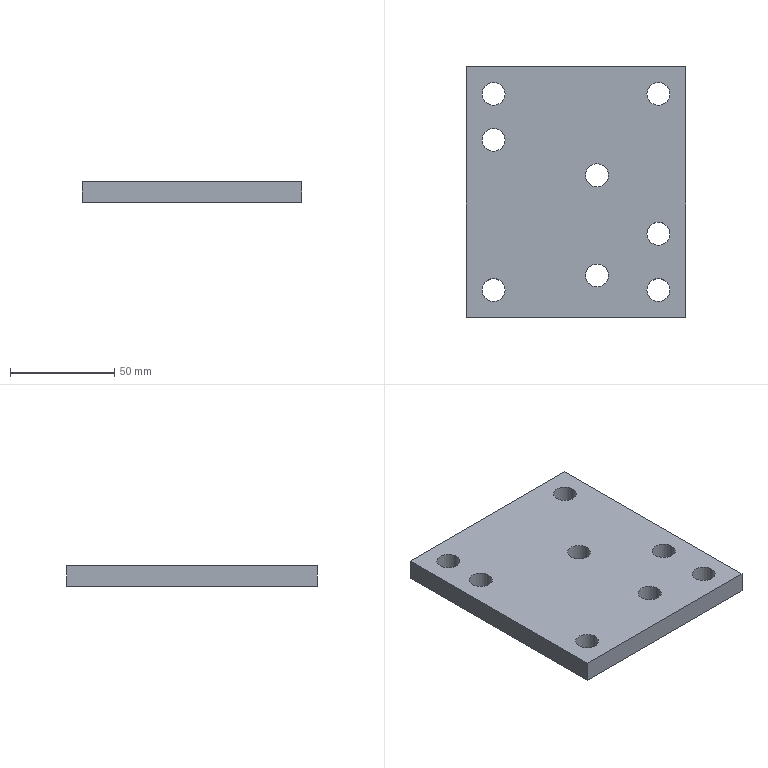Part | STEP file | PN_0044_id966_x_t | 1 solid | 14 faces | box 105 x 120 x 10 mm | volume 118397 mm3 | cylinder 8 | plane 6 | commonest cylinder face diameters 11 x8
STEP:
#1=CARTESIAN_POINT('',(-66.,8.,95.));
#2=VERTEX_POINT('',#1);
#3=CARTESIAN_POINT('',(-66.,8.,105.));
#4=VERTEX_POINT('',#3);
#5=CARTESIAN_POINT('',(-66.,8.,95.));
#6=DIRECTION('',(0.,0.,1.));
#7=VECTOR('',#6,1.);
#8=LINE('',#5,#7);
#9=EDGE_CURVE('',#2,#4,#8,.T.);
#10=ORIENTED_EDGE('',*,*,#9,.F.);
#11=CARTESIAN_POINT('',(-66.,128.,95.));
#12=VERTEX_POINT('',#11);
#13=CARTESIAN_POINT('',(-66.,-47.,95.));
#14=DIRECTION('',(0.,1.,0.));
#15=VECTOR('',#14,1.);
#16=LINE('',#13,#15);
#17=EDGE_CURVE('',#2,#12,#16,.T.);
#18=ORIENTED_EDGE('',*,*,#17,.T.);
#19=CARTESIAN_POINT('',(-66.,128.,105.));
#20=VERTEX_POINT('',#19);
#21=CARTESIAN_POINT('',(-66.,128.,95.));
#22=DIRECTION('',(0.,0.,1.));
#23=VECTOR('',#22,1.);
#24=LINE('',#21,#23);
#25=EDGE_CURVE('',#12,#20,#24,.T.);
#26=ORIENTED_EDGE('',*,*,#25,.T.);
#27=CARTESIAN_POINT('',(-66.,-47.,105.));
#28=DIRECTION('',(0.,1.,0.));
#29=VECTOR('',#28,1.);
#30=LINE('',#27,#29);
#31=EDGE_CURVE('',#4,#20,#30,.T.);
#32=ORIENTED_EDGE('',*,*,#31,.F.);
#33=EDGE_LOOP('',(#10,#18,#26,#32));
#34=FACE_OUTER_BOUND('',#33,.T.);
#35=CARTESIAN_POINT('',(-66.,-47.,95.));
#36=DIRECTION('',(1.,0.,0.));
#37=DIRECTION('',(0.,1.,0.));
#38=AXIS2_PLACEMENT_3D('',#35,#36,#37);
#39=PLANE('',#38);
#40=ADVANCED_FACE('',(#34),#39,.T.);
#41=ORIENTED_EDGE('',*,*,#25,.F.);
#42=CARTESIAN_POINT('',(-171.,128.,95.));
#43=VERTEX_POINT('',#42);
#44=CARTESIAN_POINT('',(-321.,128.,95.));
#45=DIRECTION('',(-1.,0.,0.));
#46=VECTOR('',#45,1.);
#47=LINE('',#44,#46);
#48=EDGE_CURVE('',#12,#43,#47,.T.);
#49=ORIENTED_EDGE('',*,*,#48,.T.);
#50=CARTESIAN_POINT('',(-171.,128.,105.));
#51=VERTEX_POINT('',#50);
#52=CARTESIAN_POINT('',(-171.,128.,95.));
#53=DIRECTION('',(0.,0.,1.));
#54=VECTOR('',#53,1.);
#55=LINE('',#52,#54);
#56=EDGE_CURVE('',#43,#51,#55,.T.);
#57=ORIENTED_EDGE('',*,*,#56,.T.);
#58=CARTESIAN_POINT('',(-321.,128.,105.));
#59=DIRECTION('',(-1.,0.,0.));
#60=VECTOR('',#59,1.);
#61=LINE('',#58,#60);
#62=EDGE_CURVE('',#20,#51,#61,.T.);
#63=ORIENTED_EDGE('',*,*,#62,.F.);
#64=EDGE_LOOP('',(#41,#49,#57,#63));
#65=FACE_OUTER_BOUND('',#64,.T.);
#66=CARTESIAN_POINT('',(-119.811,128.,95.));
#67=DIRECTION('',(0.,1.,0.));
#68=DIRECTION('',(-1.,0.,0.));
#69=AXIS2_PLACEMENT_3D('',#66,#67,#68);
#70=PLANE('',#69);
#71=ADVANCED_FACE('',(#65),#70,.T.);
#72=ORIENTED_EDGE('',*,*,#56,.F.);
#73=CARTESIAN_POINT('',(-171.,8.,95.));
#74=VERTEX_POINT('',#73);
#75=CARTESIAN_POINT('',(-171.,-47.,95.));
#76=DIRECTION('',(0.,-1.,0.));
#77=VECTOR('',#76,1.);
#78=LINE('',#75,#77);
#79=EDGE_CURVE('',#43,#74,#78,.T.);
#80=ORIENTED_EDGE('',*,*,#79,.T.);
#81=CARTESIAN_POINT('',(-171.,8.,105.));
#82=VERTEX_POINT('',#81);
#83=CARTESIAN_POINT('',(-171.,8.,95.));
#84=DIRECTION('',(0.,0.,1.));
#85=VECTOR('',#84,1.);
#86=LINE('',#83,#85);
#87=EDGE_CURVE('',#74,#82,#86,.T.);
#88=ORIENTED_EDGE('',*,*,#87,.T.);
#89=CARTESIAN_POINT('',(-171.,-47.,105.));
#90=DIRECTION('',(0.,-1.,0.));
#91=VECTOR('',#90,1.);
#92=LINE('',#89,#91);
#93=EDGE_CURVE('',#51,#82,#92,.T.);
#94=ORIENTED_EDGE('',*,*,#93,.F.);
#95=EDGE_LOOP('',(#72,#80,#88,#94));
#96=FACE_OUTER_BOUND('',#95,.T.);
#97=CARTESIAN_POINT('',(-171.,-47.,95.));
#98=DIRECTION('',(-1.,0.,0.));
#99=DIRECTION('',(0.,-1.,0.));
#100=AXIS2_PLACEMENT_3D('',#97,#98,#99);
#101=PLANE('',#100);
#102=ADVANCED_FACE('',(#96),#101,.T.);
#103=CARTESIAN_POINT('',(-119.811,8.,95.));
#104=DIRECTION('',(1.,0.,0.));
#105=VECTOR('',#104,1.);
#106=LINE('',#103,#105);
#107=EDGE_CURVE('',#74,#2,#106,.T.);
#108=ORIENTED_EDGE('',*,*,#107,.T.);
#109=ORIENTED_EDGE('',*,*,#9,.T.);
#110=CARTESIAN_POINT('',(-321.,8.,105.));
#111=DIRECTION('',(1.,0.,0.));
#112=VECTOR('',#111,1.);
#113=LINE('',#110,#112);
#114=EDGE_CURVE('',#82,#4,#113,.T.);
#115=ORIENTED_EDGE('',*,*,#114,.F.);
#116=ORIENTED_EDGE('',*,*,#87,.F.);
#117=EDGE_LOOP('',(#108,#109,#115,#116));
#118=FACE_OUTER_BOUND('',#117,.T.);
#119=CARTESIAN_POINT('',(-119.811,8.,95.));
#120=DIRECTION('',(0.,-1.,0.));
#121=DIRECTION('',(1.,0.,0.));
#122=AXIS2_PLACEMENT_3D('',#119,#120,#121);
#123=PLANE('',#122);
#124=ADVANCED_FACE('',(#118),#123,.T.);
#125=CARTESIAN_POINT('',(-73.5,21.,105.));
#126=VERTEX_POINT('',#125);
#127=CARTESIAN_POINT('',(-79.,21.,105.));
#128=DIRECTION('',(0.,0.,-1.));
#129=DIRECTION('',(1.,0.,0.));
#130=AXIS2_PLACEMENT_3D('',#127,#128,#129);
#131=CIRCLE('',#130,5.5);
#132=EDGE_CURVE('',#126,#126,#131,.T.);
#133=ORIENTED_EDGE('',*,*,#132,.T.);
#134=EDGE_LOOP('',(#133));
#135=FACE_BOUND('',#134,.T.);
#136=CARTESIAN_POINT('',(-73.5,48.,105.));
#137=VERTEX_POINT('',#136);
#138=CARTESIAN_POINT('',(-79.,48.,105.));
#139=DIRECTION('',(0.,0.,-1.));
#140=DIRECTION('',(1.,0.,0.));
#141=AXIS2_PLACEMENT_3D('',#138,#139,#140);
#142=CIRCLE('',#141,5.5);
#143=EDGE_CURVE('',#137,#137,#142,.T.);
#144=ORIENTED_EDGE('',*,*,#143,.T.);
#145=EDGE_LOOP('',(#144));
#146=FACE_BOUND('',#145,.T.);
#147=CARTESIAN_POINT('',(-163.5,21.,105.));
#148=VERTEX_POINT('',#147);
#149=CARTESIAN_POINT('',(-158.,21.,105.));
#150=DIRECTION('',(0.,0.,1.));
#151=DIRECTION('',(-1.,0.,0.));
#152=AXIS2_PLACEMENT_3D('',#149,#150,#151);
#153=CIRCLE('',#152,5.5);
#154=EDGE_CURVE('',#148,#148,#153,.T.);
#155=ORIENTED_EDGE('',*,*,#154,.F.);
#156=EDGE_LOOP('',(#155));
#157=FACE_BOUND('',#156,.T.);
#158=CARTESIAN_POINT('',(-73.5,115.,105.));
#159=VERTEX_POINT('',#158);
#160=CARTESIAN_POINT('',(-79.,115.,105.));
#161=DIRECTION('',(0.,0.,1.));
#162=DIRECTION('',(1.,0.,0.));
#163=AXIS2_PLACEMENT_3D('',#160,#161,#162);
#164=CIRCLE('',#163,5.5);
#165=EDGE_CURVE('',#159,#159,#164,.T.);
#166=ORIENTED_EDGE('',*,*,#165,.F.);
#167=EDGE_LOOP('',(#166));
#168=FACE_BOUND('',#167,.T.);
#169=CARTESIAN_POINT('',(-163.5,115.,105.));
#170=VERTEX_POINT('',#169);
#171=CARTESIAN_POINT('',(-158.,115.,105.));
#172=DIRECTION('',(0.,0.,-1.));
#173=DIRECTION('',(-1.,0.,0.));
#174=AXIS2_PLACEMENT_3D('',#171,#172,#173);
#175=CIRCLE('',#174,5.5);
#176=EDGE_CURVE('',#170,#170,#175,.T.);
#177=ORIENTED_EDGE('',*,*,#176,.T.);
#178=EDGE_LOOP('',(#177));
#179=FACE_BOUND('',#178,.T.);
#180=CARTESIAN_POINT('',(-163.5,93.,105.));
#181=VERTEX_POINT('',#180);
#182=CARTESIAN_POINT('',(-158.,93.,105.));
#183=DIRECTION('',(0.,0.,-1.));
#184=DIRECTION('',(-1.,0.,0.));
#185=AXIS2_PLACEMENT_3D('',#182,#183,#184);
#186=CIRCLE('',#185,5.5);
#187=EDGE_CURVE('',#181,#181,#186,.T.);
#188=ORIENTED_EDGE('',*,*,#187,.T.);
#189=EDGE_LOOP('',(#188));
#190=FACE_BOUND('',#189,.T.);
#191=CARTESIAN_POINT('',(-113.99,76.,105.));
#192=VERTEX_POINT('',#191);
#193=CARTESIAN_POINT('',(-108.49,76.,105.));
#194=DIRECTION('',(0.,0.,-1.));
#195=DIRECTION('',(-1.,0.,0.));
#196=AXIS2_PLACEMENT_3D('',#193,#194,#195);
#197=CIRCLE('',#196,5.5);
#198=EDGE_CURVE('',#192,#192,#197,.T.);
#199=ORIENTED_EDGE('',*,*,#198,.T.);
#200=EDGE_LOOP('',(#199));
#201=FACE_BOUND('',#200,.T.);
#202=CARTESIAN_POINT('',(-113.99,28.,105.));
#203=VERTEX_POINT('',#202);
#204=CARTESIAN_POINT('',(-108.49,28.,105.));
#205=DIRECTION('',(0.,0.,-1.));
#206=DIRECTION('',(-1.,0.,0.));
#207=AXIS2_PLACEMENT_3D('',#204,#205,#206);
#208=CIRCLE('',#207,5.5);
#209=EDGE_CURVE('',#203,#203,#208,.T.);
#210=ORIENTED_EDGE('',*,*,#209,.T.);
#211=EDGE_LOOP('',(#210));
#212=FACE_BOUND('',#211,.T.);
#213=ORIENTED_EDGE('',*,*,#93,.T.);
#214=ORIENTED_EDGE('',*,*,#114,.T.);
#215=ORIENTED_EDGE('',*,*,#31,.T.);
#216=ORIENTED_EDGE('',*,*,#62,.T.);
#217=EDGE_LOOP('',(#213,#214,#215,#216));
#218=FACE_BOUND('',#217,.T.);
#219=CARTESIAN_POINT('',(-321.,-47.,105.));
#220=DIRECTION('',(0.,0.,1.));
#221=DIRECTION('',(1.,0.,0.));
#222=AXIS2_PLACEMENT_3D('',#219,#220,#221);
#223=PLANE('',#222);
#224=ADVANCED_FACE('',(#135,#146,#157,#168,#179,#190,#201,#212,#218),#223,.T.);
#225=CARTESIAN_POINT('',(-73.5,21.,95.));
#226=VERTEX_POINT('',#225);
#227=CARTESIAN_POINT('',(-79.,21.,95.));
#228=DIRECTION('',(0.,0.,1.));
#229=DIRECTION('',(1.,0.,0.));
#230=AXIS2_PLACEMENT_3D('',#227,#228,#229);
#231=CIRCLE('',#230,5.5);
#232=EDGE_CURVE('',#226,#226,#231,.T.);
#233=ORIENTED_EDGE('',*,*,#232,.T.);
#234=EDGE_LOOP('',(#233));
#235=FACE_BOUND('',#234,.T.);
#236=CARTESIAN_POINT('',(-73.5,48.,95.));
#237=VERTEX_POINT('',#236);
#238=CARTESIAN_POINT('',(-79.,48.,95.));
#239=DIRECTION('',(0.,0.,1.));
#240=DIRECTION('',(1.,0.,0.));
#241=AXIS2_PLACEMENT_3D('',#238,#239,#240);
#242=CIRCLE('',#241,5.5);
#243=EDGE_CURVE('',#237,#237,#242,.T.);
#244=ORIENTED_EDGE('',*,*,#243,.T.);
#245=EDGE_LOOP('',(#244));
#246=FACE_BOUND('',#245,.T.);
#247=CARTESIAN_POINT('',(-152.5,21.,95.));
#248=VERTEX_POINT('',#247);
#249=CARTESIAN_POINT('',(-158.,21.,95.));
#250=DIRECTION('',(0.,0.,1.));
#251=DIRECTION('',(1.,0.,0.));
#252=AXIS2_PLACEMENT_3D('',#249,#250,#251);
#253=CIRCLE('',#252,5.5);
#254=EDGE_CURVE('',#248,#248,#253,.T.);
#255=ORIENTED_EDGE('',*,*,#254,.T.);
#256=EDGE_LOOP('',(#255));
#257=FACE_BOUND('',#256,.T.);
#258=CARTESIAN_POINT('',(-73.5,115.,95.));
#259=VERTEX_POINT('',#258);
#260=CARTESIAN_POINT('',(-79.,115.,95.));
#261=DIRECTION('',(0.,0.,1.));
#262=DIRECTION('',(1.,0.,0.));
#263=AXIS2_PLACEMENT_3D('',#260,#261,#262);
#264=CIRCLE('',#263,5.5);
#265=EDGE_CURVE('',#259,#259,#264,.T.);
#266=ORIENTED_EDGE('',*,*,#265,.T.);
#267=EDGE_LOOP('',(#266));
#268=FACE_BOUND('',#267,.T.);
#269=CARTESIAN_POINT('',(-152.5,115.,95.));
#270=VERTEX_POINT('',#269);
#271=CARTESIAN_POINT('',(-158.,115.,95.));
#272=DIRECTION('',(0.,0.,1.));
#273=DIRECTION('',(1.,0.,0.));
#274=AXIS2_PLACEMENT_3D('',#271,#272,#273);
#275=CIRCLE('',#274,5.5);
#276=EDGE_CURVE('',#270,#270,#275,.T.);
#277=ORIENTED_EDGE('',*,*,#276,.T.);
#278=EDGE_LOOP('',(#277));
#279=FACE_BOUND('',#278,.T.);
#280=CARTESIAN_POINT('',(-163.5,93.,95.));
#281=VERTEX_POINT('',#280);
#282=CARTESIAN_POINT('',(-158.,93.,95.));
#283=DIRECTION('',(0.,0.,1.));
#284=DIRECTION('',(-1.,0.,0.));
#285=AXIS2_PLACEMENT_3D('',#282,#283,#284);
#286=CIRCLE('',#285,5.5);
#287=EDGE_CURVE('',#281,#281,#286,.T.);
#288=ORIENTED_EDGE('',*,*,#287,.T.);
#289=EDGE_LOOP('',(#288));
#290=FACE_BOUND('',#289,.T.);
#291=CARTESIAN_POINT('',(-102.99,76.,95.));
#292=VERTEX_POINT('',#291);
#293=CARTESIAN_POINT('',(-108.49,76.,95.));
#294=DIRECTION('',(0.,0.,1.));
#295=DIRECTION('',(1.,0.,0.));
#296=AXIS2_PLACEMENT_3D('',#293,#294,#295);
#297=CIRCLE('',#296,5.5);
#298=EDGE_CURVE('',#292,#292,#297,.T.);
#299=ORIENTED_EDGE('',*,*,#298,.T.);
#300=EDGE_LOOP('',(#299));
#301=FACE_BOUND('',#300,.T.);
#302=CARTESIAN_POINT('',(-102.99,28.,95.));
#303=VERTEX_POINT('',#302);
#304=CARTESIAN_POINT('',(-108.49,28.,95.));
#305=DIRECTION('',(0.,0.,1.));
#306=DIRECTION('',(1.,0.,0.));
#307=AXIS2_PLACEMENT_3D('',#304,#305,#306);
#308=CIRCLE('',#307,5.5);
#309=EDGE_CURVE('',#303,#303,#308,.T.);
#310=ORIENTED_EDGE('',*,*,#309,.T.);
#311=EDGE_LOOP('',(#310));
#312=FACE_BOUND('',#311,.T.);
#313=ORIENTED_EDGE('',*,*,#79,.F.);
#314=ORIENTED_EDGE('',*,*,#48,.F.);
#315=ORIENTED_EDGE('',*,*,#17,.F.);
#316=ORIENTED_EDGE('',*,*,#107,.F.);
#317=EDGE_LOOP('',(#313,#314,#315,#316));
#318=FACE_BOUND('',#317,.T.);
#319=CARTESIAN_POINT('',(-321.,-47.,95.));
#320=DIRECTION('',(0.,0.,1.));
#321=DIRECTION('',(1.,0.,0.));
#322=AXIS2_PLACEMENT_3D('',#319,#320,#321);
#323=PLANE('',#322);
#324=ADVANCED_FACE('',(#235,#246,#257,#268,#279,#290,#301,#312,#318),#323,.F.);
#325=ORIENTED_EDGE('',*,*,#209,.F.);
#326=EDGE_LOOP('',(#325));
#327=FACE_BOUND('',#326,.T.);
#328=ORIENTED_EDGE('',*,*,#309,.F.);
#329=EDGE_LOOP('',(#328));
#330=FACE_BOUND('',#329,.T.);
#331=CARTESIAN_POINT('',(-108.49,28.,105.));
#332=DIRECTION('',(0.,0.,-1.));
#333=DIRECTION('',(-1.,0.,0.));
#334=AXIS2_PLACEMENT_3D('',#331,#332,#333);
#335=CYLINDRICAL_SURFACE('',#334,5.5);
#336=ADVANCED_FACE('',(#327,#330),#335,.F.);
#337=ORIENTED_EDGE('',*,*,#198,.F.);
#338=EDGE_LOOP('',(#337));
#339=FACE_BOUND('',#338,.T.);
#340=ORIENTED_EDGE('',*,*,#298,.F.);
#341=EDGE_LOOP('',(#340));
#342=FACE_BOUND('',#341,.T.);
#343=CARTESIAN_POINT('',(-108.49,76.,105.));
#344=DIRECTION('',(0.,0.,-1.));
#345=DIRECTION('',(-1.,0.,0.));
#346=AXIS2_PLACEMENT_3D('',#343,#344,#345);
#347=CYLINDRICAL_SURFACE('',#346,5.5);
#348=ADVANCED_FACE('',(#339,#342),#347,.F.);
#349=ORIENTED_EDGE('',*,*,#287,.F.);
#350=EDGE_LOOP('',(#349));
#351=FACE_BOUND('',#350,.T.);
#352=ORIENTED_EDGE('',*,*,#187,.F.);
#353=EDGE_LOOP('',(#352));
#354=FACE_BOUND('',#353,.T.);
#355=CARTESIAN_POINT('',(-158.,93.,105.));
#356=DIRECTION('',(0.,0.,-1.));
#357=DIRECTION('',(-1.,0.,0.));
#358=AXIS2_PLACEMENT_3D('',#355,#356,#357);
#359=CYLINDRICAL_SURFACE('',#358,5.5);
#360=ADVANCED_FACE('',(#351,#354),#359,.F.);
#361=ORIENTED_EDGE('',*,*,#176,.F.);
#362=EDGE_LOOP('',(#361));
#363=FACE_BOUND('',#362,.T.);
#364=ORIENTED_EDGE('',*,*,#276,.F.);
#365=EDGE_LOOP('',(#364));
#366=FACE_BOUND('',#365,.T.);
#367=CARTESIAN_POINT('',(-158.,115.,105.));
#368=DIRECTION('',(0.,0.,-1.));
#369=DIRECTION('',(-1.,0.,0.));
#370=AXIS2_PLACEMENT_3D('',#367,#368,#369);
#371=CYLINDRICAL_SURFACE('',#370,5.5);
#372=ADVANCED_FACE('',(#363,#366),#371,.F.);
#373=ORIENTED_EDGE('',*,*,#165,.T.);
#374=EDGE_LOOP('',(#373));
#375=FACE_BOUND('',#374,.T.);
#376=ORIENTED_EDGE('',*,*,#265,.F.);
#377=EDGE_LOOP('',(#376));
#378=FACE_BOUND('',#377,.T.);
#379=CARTESIAN_POINT('',(-79.,115.,105.));
#380=DIRECTION('',(0.,0.,-1.));
#381=DIRECTION('',(1.,0.,0.));
#382=AXIS2_PLACEMENT_3D('',#379,#380,#381);
#383=CYLINDRICAL_SURFACE('',#382,5.5);
#384=ADVANCED_FACE('',(#375,#378),#383,.F.);
#385=ORIENTED_EDGE('',*,*,#154,.T.);
#386=EDGE_LOOP('',(#385));
#387=FACE_BOUND('',#386,.T.);
#388=ORIENTED_EDGE('',*,*,#254,.F.);
#389=EDGE_LOOP('',(#388));
#390=FACE_BOUND('',#389,.T.);
#391=CARTESIAN_POINT('',(-158.,21.,105.));
#392=DIRECTION('',(0.,0.,-1.));
#393=DIRECTION('',(-1.,0.,0.));
#394=AXIS2_PLACEMENT_3D('',#391,#392,#393);
#395=CYLINDRICAL_SURFACE('',#394,5.5);
#396=ADVANCED_FACE('',(#387,#390),#395,.F.);
#397=ORIENTED_EDGE('',*,*,#243,.F.);
#398=EDGE_LOOP('',(#397));
#399=FACE_BOUND('',#398,.T.);
#400=ORIENTED_EDGE('',*,*,#143,.F.);
#401=EDGE_LOOP('',(#400));
#402=FACE_BOUND('',#401,.T.);
#403=CARTESIAN_POINT('',(-79.,48.,105.));
#404=DIRECTION('',(0.,0.,-1.));
#405=DIRECTION('',(1.,0.,0.));
#406=AXIS2_PLACEMENT_3D('',#403,#404,#405);
#407=CYLINDRICAL_SURFACE('',#406,5.5);
#408=ADVANCED_FACE('',(#399,#402),#407,.F.);
#409=ORIENTED_EDGE('',*,*,#132,.F.);
#410=EDGE_LOOP('',(#409));
#411=FACE_BOUND('',#410,.T.);
#412=ORIENTED_EDGE('',*,*,#232,.F.);
#413=EDGE_LOOP('',(#412));
#414=FACE_BOUND('',#413,.T.);
#415=CARTESIAN_POINT('',(-79.,21.,105.));
#416=DIRECTION('',(0.,0.,-1.));
#417=DIRECTION('',(1.,0.,0.));
#418=AXIS2_PLACEMENT_3D('',#415,#416,#417);
#419=CYLINDRICAL_SURFACE('',#418,5.5);
#420=ADVANCED_FACE('',(#411,#414),#419,.F.);
#421=CLOSED_SHELL('',(#40,#71,#102,#124,#224,#324,#336,#348,#360,#372,#384,#396,#408,#420));
#422=MANIFOLD_SOLID_BREP('',#421);
#423=(LENGTH_UNIT()NAMED_UNIT(*)SI_UNIT(.MILLI.,.METRE.));
#424=UNCERTAINTY_MEASURE_WITH_UNIT(LENGTH_MEASURE(0.00002),#423,'','');
#425=(NAMED_UNIT(*)PLANE_ANGLE_UNIT()SI_UNIT($,.RADIAN.));
#426=PLANE_ANGLE_MEASURE_WITH_UNIT(PLANE_ANGLE_MEASURE(0.01745),#425);
#427=DIMENSIONAL_EXPONENTS(0.,0.,0.,0.,0.,0.,0.);
#428=(CONVERSION_BASED_UNIT('DEGREE',#426)NAMED_UNIT(#427)PLANE_ANGLE_UNIT());
#429=(NAMED_UNIT(*)SI_UNIT($,.STERADIAN.)SOLID_ANGLE_UNIT());
#430=(GEOMETRIC_REPRESENTATION_CONTEXT(3)GLOBAL_UNCERTAINTY_ASSIGNED_CONTEXT((#424))GLOBAL_UNIT_ASSIGNED_CONTEXT((#423,#428,#429))REPRESENTATION_CONTEXT('',''));
#431=ADVANCED_BREP_SHAPE_REPRESENTATION('',(#422),#430);